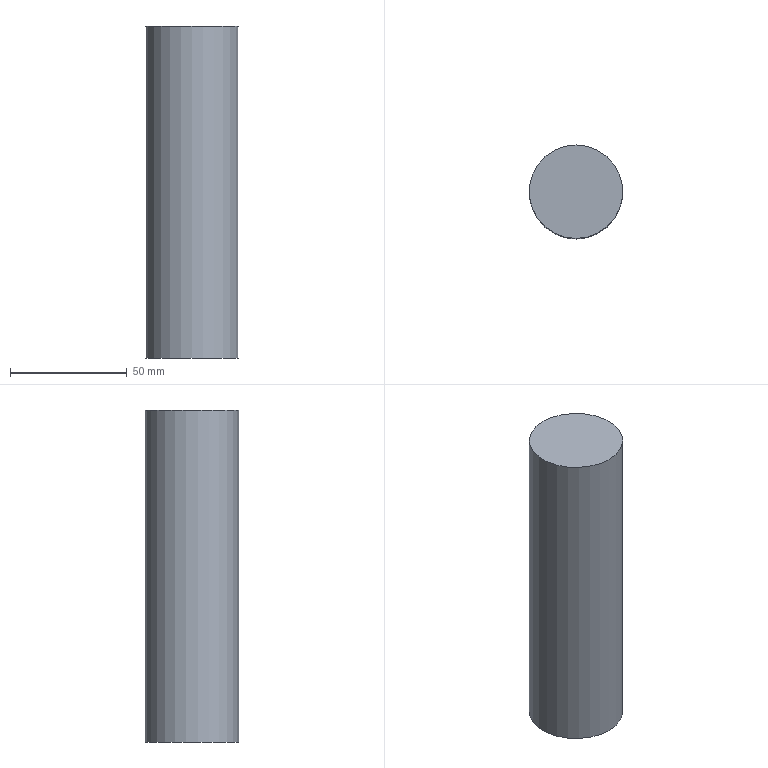Part | NX | features solid 2 | 1 solid | 3 faces | box 40 x 40 x 142 mm | volume 178442 mm3 | plane 2 | cylinder 1 | commonest cylinder face diameters 40 x1
STEP:
#1=CARTESIAN_POINT('',(255.,10.,-252.));
#2=VERTEX_POINT('',#1);
#3=CARTESIAN_POINT('',(255.,-10.,-252.));
#4=DIRECTION('',(0.,0.,-1.));
#5=DIRECTION('',(0.,1.,0.));
#6=AXIS2_PLACEMENT_3D('',#3,#4,#5);
#7=CIRCLE('',#6,20.);
#8=EDGE_CURVE('',#2,#2,#7,.T.);
#9=ORIENTED_EDGE('',*,*,#8,.F.);
#10=EDGE_LOOP('',(#9));
#11=FACE_BOUND('',#10,.T.);
#12=CARTESIAN_POINT('',(255.,10.,-110.));
#13=VERTEX_POINT('',#12);
#14=CARTESIAN_POINT('',(255.,-10.,-110.));
#15=DIRECTION('',(0.,0.,-1.));
#16=DIRECTION('',(0.,1.,0.));
#17=AXIS2_PLACEMENT_3D('',#14,#15,#16);
#18=CIRCLE('',#17,20.);
#19=EDGE_CURVE('',#13,#13,#18,.T.);
#20=ORIENTED_EDGE('',*,*,#19,.T.);
#21=EDGE_LOOP('',(#20));
#22=FACE_BOUND('',#21,.T.);
#23=CARTESIAN_POINT('',(255.,-10.,-252.));
#24=DIRECTION('',(0.,0.,1.));
#25=DIRECTION('',(0.,1.,0.));
#26=AXIS2_PLACEMENT_3D('',#23,#24,#25);
#27=CYLINDRICAL_SURFACE('',#26,20.);
#28=ADVANCED_FACE('',(#11,#22),#27,.T.);
#29=ORIENTED_EDGE('',*,*,#8,.T.);
#30=EDGE_LOOP('',(#29));
#31=FACE_BOUND('',#30,.T.);
#32=CARTESIAN_POINT('',(255.,-10.,-252.));
#33=DIRECTION('',(0.,0.,-1.));
#34=DIRECTION('',(0.,-1.,0.));
#35=AXIS2_PLACEMENT_3D('',#32,#33,#34);
#36=PLANE('',#35);
#37=ADVANCED_FACE('',(#31),#36,.T.);
#38=ORIENTED_EDGE('',*,*,#19,.F.);
#39=EDGE_LOOP('',(#38));
#40=FACE_BOUND('',#39,.T.);
#41=CARTESIAN_POINT('',(255.,-10.,-110.));
#42=DIRECTION('',(0.,0.,-1.));
#43=DIRECTION('',(0.,-1.,0.));
#44=AXIS2_PLACEMENT_3D('',#41,#42,#43);
#45=PLANE('',#44);
#46=ADVANCED_FACE('',(#40),#45,.F.);
#47=CLOSED_SHELL('',(#28,#37,#46));
#48=MANIFOLD_SOLID_BREP('',#47);
#49=(LENGTH_UNIT()NAMED_UNIT(*)SI_UNIT(.MILLI.,.METRE.));
#50=UNCERTAINTY_MEASURE_WITH_UNIT(LENGTH_MEASURE(0.00001),#49,'','');
#51=(NAMED_UNIT(*)PLANE_ANGLE_UNIT()SI_UNIT($,.RADIAN.));
#52=(NAMED_UNIT(*)SI_UNIT($,.STERADIAN.)SOLID_ANGLE_UNIT());
#53=(GEOMETRIC_REPRESENTATION_CONTEXT(3)GLOBAL_UNCERTAINTY_ASSIGNED_CONTEXT((#50))GLOBAL_UNIT_ASSIGNED_CONTEXT((#49,#51,#52))REPRESENTATION_CONTEXT('',''));
#54=ADVANCED_BREP_SHAPE_REPRESENTATION('',(#48),#53);